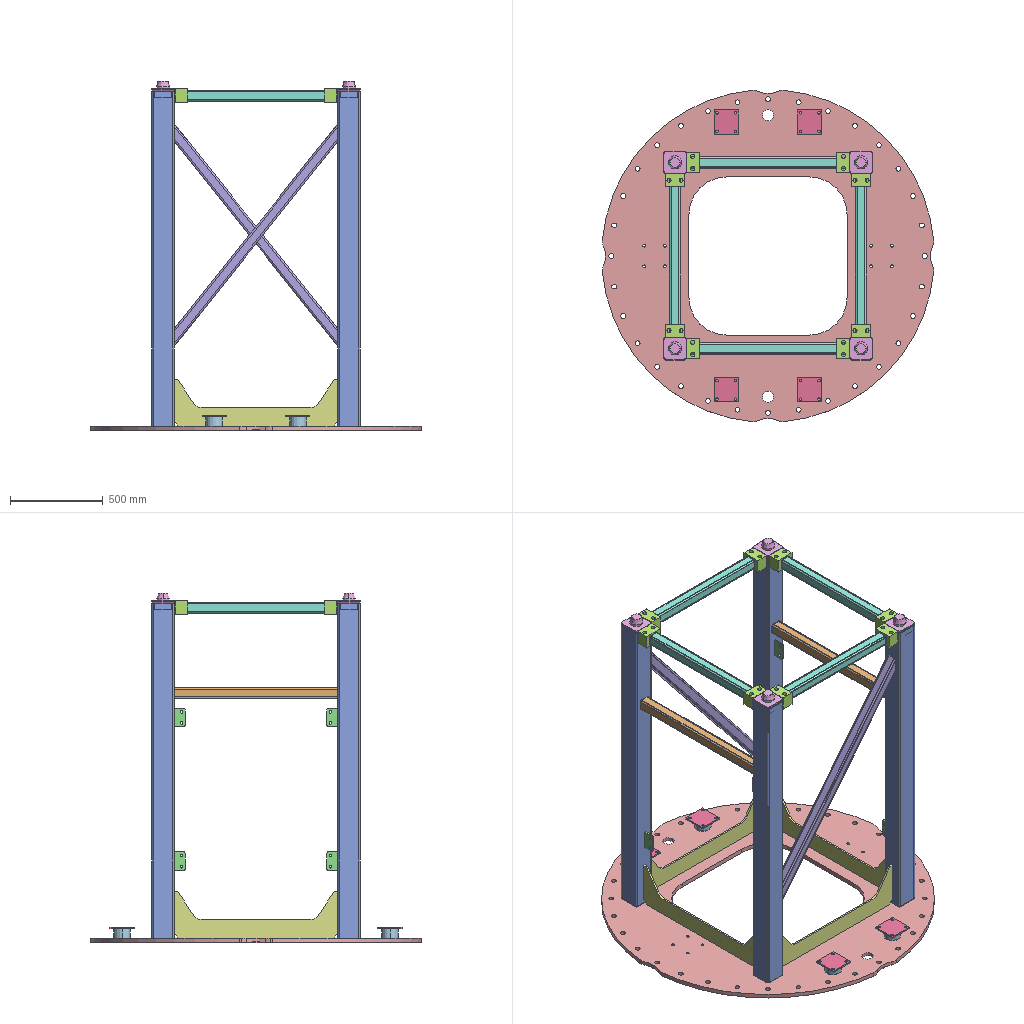Assembly | SolidWorks | 14 different items | 47 placed | box 1782 x 1782 x 1880 mm
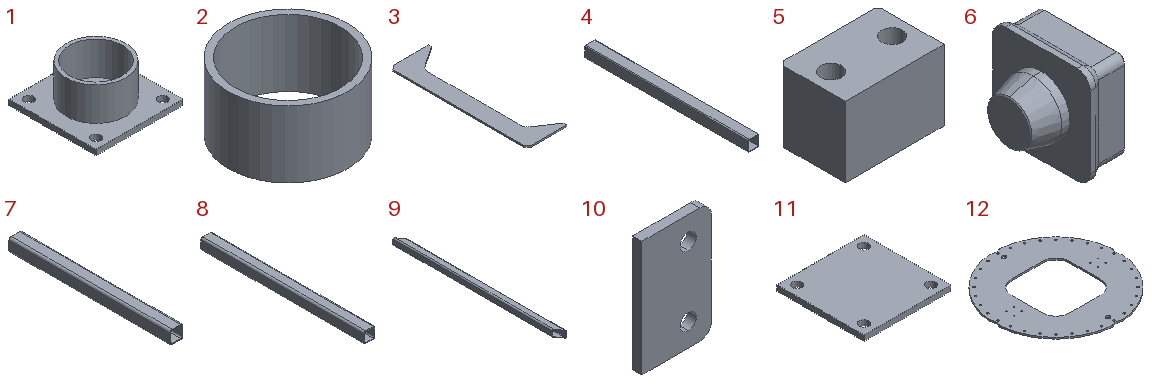Parts list (item | name | quantity | parent item | size | volume | features):
1 | (subassembly) | x4 | - | 130 x 130 x 58 mm | 196247 mm3 | features CompositeCurve 1
2 | - | x4 | in 1 | 89 x 89 x 50 mm | 65973 mm3 | features Extrusion 1
3 | - | x4 | - | 250 x 880 x 10 mm | 1085939 mm3 | features Chamfer 1, Extrusion 1, Fillet 1
4 | - | x4 | - | 120 x 1800 x 120 mm | 4795009 mm3 | features Extrusion 1
5 | - | x8 | - | 105 x 70 x 75 mm | 492355 mm3 | features Extrusion 1
6 | - | x4 | - | 90 x 120 x 120 mm | 737957 mm3 | features Chamfer 3, ICE 2, Revolution 1
7 | - | x4 | - | 60 x 740 x 60 mm | 622386 mm3 | features Extrusion 1
8 | - | x2 | - | 60 x 880 x 60 mm | 740134 mm3 | features Extrusion 1
9 | - | x2 | - | 60 x 1484 x 60 mm | 1185056 mm3 | features Extrusion 1, ICE 1
10 | - | x4 | - | 60 x 8 x 100 mm | 45194 mm3 | features Extrusion 1
11 | - | x4 | in 1 | 130 x 130 x 8 mm | 130274 mm3 | features Extrusion 1
12 | - | x1 | - | 1782 x 1782 x 25 mm | 40028246 mm3 | features ICE 2, Extrusion 1
13 | XZT16B.02.01.11 Tower Base Lower Rib Plate2 | x1 | - | - | - | -
14 | XZT16B.02.01.12 Air Compressor Mounting Angle Bracket | x1 | - | - | - | -
Mates (type | each side: item.copy, entity, surface, feature):
In the top assembly
Coincident | 12.1 face plane Boss-Extrude1 | 4.1 face plane Boss-Extrude1
Coincident | 4.1 face plane Boss-Extrude1 | 6.1 face plane Boss-Extrude1
Coincident | 4.1 face plane Boss-Extrude1 | 6.1 face plane Boss-Extrude2 | 2 times
Symmetric | 7.1 face plane Boss-Extrude1 | 7.1 face plane Boss-Extrude1 | assembly plane
Coincident | 9.1 face plane Cut-Extrude1 | 4.2 face plane Boss-Extrude1
Parallel | 9.1 face plane Boss-Extrude1 | 4.2 face plane Boss-Extrude1
Coincident | 12.1 face plane Boss-Extrude1 | 3.1 face plane Boss-Extrude1
Parallel | 3.1 face plane Boss-Extrude1 | 4.3 face plane Boss-Extrude1
Symmetric | 3.1 face plane Boss-Extrude1 | 3.1 face plane Boss-Extrude1 | assembly plane
Coincident | 4.1 face plane Boss-Extrude1 | 3.1 face plane Boss-Extrude1
Coincident | 8.1 face plane Boss-Extrude1 | 4.3 face plane Boss-Extrude1
Coincident | 7.2 face plane Boss-Extrude1 | 8.1 face plane Boss-Extrude1
Coincident | 10.1 face plane Boss-Extrude1 | 4.3 face plane Boss-Extrude1
DistanceDim | 8.1 face plane Boss-Extrude1 | 10.1 face plane Boss-Extrude1
Coincident | 4.2 face plane Boss-Extrude1 | 10.2 face plane Boss-Extrude1
DistanceDim | 10.1 face plane Boss-Extrude1 | 10.2 face plane Boss-Extrude1
Coincident | 9.1 face plane Boss-Extrude1 | 7.3 face plane Boss-Extrude1
Coincident | 12.1 face plane Boss-Extrude1 | 2.1 face plane Boss-Extrude1
DistanceDim | 2.1 face cylinder Boss-Extrude1 | assembly plane | 2 times
Perpendicular | 3.1 face plane Boss-Extrude1 | 11.1 face plane Boss-Extrude1
DistanceDim | 10.1 face plane Boss-Extrude1 | 4.2 face plane Boss-Extrude1
DistanceDim | 10.2 face plane Boss-Extrude1 | 4.3 face plane Boss-Extrude1
DistanceDim | 9.1 edge | 5.1 face plane Boss-Extrude1
Coincident | 4.1 face plane Boss-Extrude1 | 5.2 face plane Boss-Extrude1
Coincident | 5.2 face plane Boss-Extrude1 | 6.1 face plane Boss-Extrude1
Width | 5.2 face plane Boss-Extrude1 | 5.2 face plane Boss-Extrude1 | 6.1 face plane Boss-Extrude1 | 6.1 face plane Boss-Extrude1
Coincident | 4.1 face plane Boss-Extrude1 | 5.3 face plane Boss-Extrude1
Width | 5.3 face plane Boss-Extrude1 | 5.3 face plane Boss-Extrude1 | 6.1 face plane Boss-Extrude1 | 6.1 face plane Boss-Extrude1
Coincident | 5.3 face plane Boss-Extrude1 | 5.2 face plane Boss-Extrude1
Coincident | 5.3 face plane Boss-Extrude1 | 7.1 face plane Boss-Extrude1
DistanceDim | 7.1 face plane Boss-Extrude1 | 5.3 face plane Boss-Extrude1
Coincident | 5.4 face plane Boss-Extrude1 | 7.1 face plane Boss-Extrude1
Coincident | 5.5 face plane Boss-Extrude1 | 7.2 face plane Boss-Extrude1
Coincident | 5.6 face plane Boss-Extrude1 | 7.2 face plane Boss-Extrude1
Coincident | 7.2 face plane Boss-Extrude1 | 7.1 face plane Boss-Extrude1
DistanceDim | 7.2 face plane Boss-Extrude1 | 5.5 face plane Boss-Extrude1
DistanceDim | 8.2 face plane Boss-Extrude1 | 5.2 face plane Boss-Extrude1
In subassembly 1
Coincident | 11.2 face plane Boss-Extrude1 | 2.2 edge
DistanceDim | 2.2 face cylinder Boss-Extrude1 | 11.2 face plane Boss-Extrude1 | 2 times